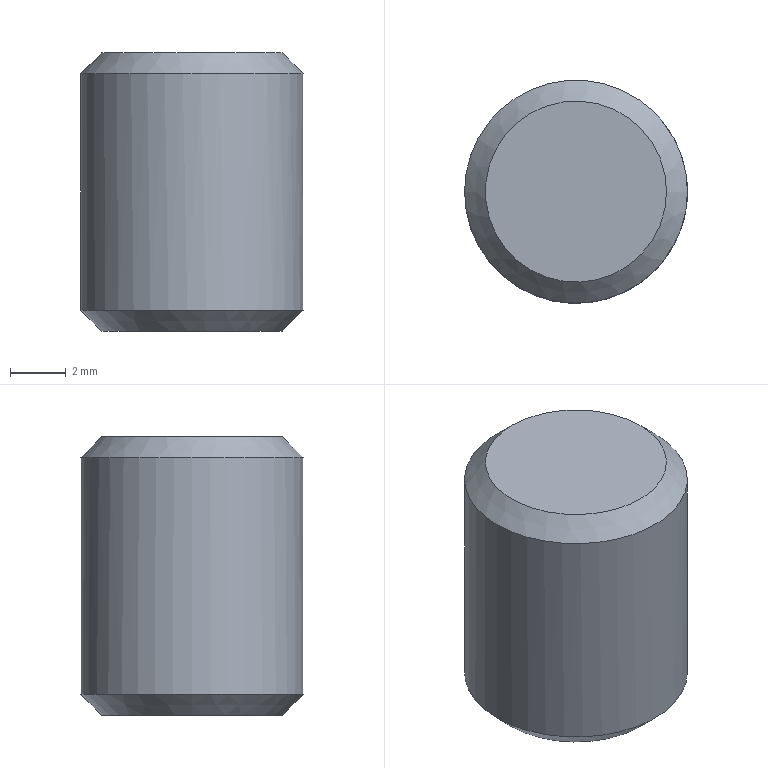Part | STEP file | 1 solid | 12 faces | box 8 x 8 x 10 mm | volume 413.018 mm3 | plane 9 | cone 2 | cylinder 1 | commonest cylinder face diameters 8 x1
STEP:
#1=CARTESIAN_POINT('',(0.,0.,0.));
#2=DIRECTION('',(0.,0.,1.));
#3=DIRECTION('',(1.,0.,0.));
#4=AXIS2_PLACEMENT_3D('',#1,#2,#3);
#5=CARTESIAN_POINT('',(1479.84,472.48,-145.381));
#6=VERTEX_POINT('',#5);
#7=CARTESIAN_POINT('',(1483.09,472.48,-145.381));
#8=DIRECTION('',(0.,0.,-1.));
#9=DIRECTION('',(-1.,0.,0.));
#10=AXIS2_PLACEMENT_3D('',#7,#8,#9);
#11=CIRCLE('',#10,3.25);
#12=CARTESIAN_POINT('',(1483.09,472.48,-145.381));
#13=DIRECTION('',(0.,0.,-1.));
#14=DIRECTION('',(-1.,0.,0.));
#15=AXIS2_PLACEMENT_3D('',#12,#13,#14);
#16=PLANE('',#15);
#17=CARTESIAN_POINT('',(0.,0.));
#18=DIRECTION('',(1.,0.));
#19=AXIS2_PLACEMENT_2D('',#17,#18);
#20=CIRCLE('',#19,3.25);
#21=(GEOMETRIC_REPRESENTATION_CONTEXT(2)PARAMETRIC_REPRESENTATION_CONTEXT()REPRESENTATION_CONTEXT('',''));
#22=DEFINITIONAL_REPRESENTATION('',(#20),#21);
#23=PCURVE('',#16,#22);
#24=CARTESIAN_POINT('',(1483.09,472.48,-144.631));
#25=DIRECTION('',(0.,0.,1.));
#26=DIRECTION('',(1.,0.,0.));
#27=AXIS2_PLACEMENT_3D('',#24,#25,#26);
#28=CONICAL_SURFACE('',#27,4.,0.7854);
#29=CARTESIAN_POINT('',(9.425,-0.75));
#30=DIRECTION('',(-1.,0.));
#31=VECTOR('',#30,1.);
#32=LINE('',#29,#31);
#33=(GEOMETRIC_REPRESENTATION_CONTEXT(2)PARAMETRIC_REPRESENTATION_CONTEXT()REPRESENTATION_CONTEXT('',''));
#34=DEFINITIONAL_REPRESENTATION('',(#32),#33);
#35=PCURVE('',#28,#34);
#36=SURFACE_CURVE('',#11,(#23,#35),.PCURVE_S1.);
#37=EDGE_CURVE('',#6,#6,#36,.T.);
#38=ORIENTED_EDGE('',*,*,#37,.T.);
#39=EDGE_LOOP('',(#38));
#40=FACE_BOUND('',#39,.T.);
#41=CARTESIAN_POINT('',(1485.19,471.268,-145.381));
#42=VERTEX_POINT('',#41);
#43=CARTESIAN_POINT('',(1483.09,470.056,-145.381));
#44=VERTEX_POINT('',#43);
#45=CARTESIAN_POINT('',(1485.19,471.268,-145.381));
#46=DIRECTION('',(-0.866,-0.5,0.));
#47=VECTOR('',#46,1.);
#48=LINE('',#45,#47);
#49=CARTESIAN_POINT('',(-2.1,-1.212));
#50=DIRECTION('',(0.866,-0.5));
#51=VECTOR('',#50,1.);
#52=LINE('',#49,#51);
#53=(GEOMETRIC_REPRESENTATION_CONTEXT(2)PARAMETRIC_REPRESENTATION_CONTEXT()REPRESENTATION_CONTEXT('',''));
#54=DEFINITIONAL_REPRESENTATION('',(#52),#53);
#55=PCURVE('',#16,#54);
#56=CARTESIAN_POINT('',(1485.19,471.268,-95.881));
#57=DIRECTION('',(0.5,-0.866,0.));
#58=DIRECTION('',(-0.866,-0.5,0.));
#59=AXIS2_PLACEMENT_3D('',#56,#57,#58);
#60=PLANE('',#59);
#61=CARTESIAN_POINT('',(0.,49.5));
#62=DIRECTION('',(1.,0.));
#63=VECTOR('',#62,1.);
#64=LINE('',#61,#63);
#65=(GEOMETRIC_REPRESENTATION_CONTEXT(2)PARAMETRIC_REPRESENTATION_CONTEXT()REPRESENTATION_CONTEXT('',''));
#66=DEFINITIONAL_REPRESENTATION('',(#64),#65);
#67=PCURVE('',#60,#66);
#68=SURFACE_CURVE('',#48,(#55,#67),.PCURVE_S1.);
#69=EDGE_CURVE('',#42,#44,#68,.T.);
#70=ORIENTED_EDGE('',*,*,#69,.F.);
#71=CARTESIAN_POINT('',(1485.19,473.693,-145.381));
#72=VERTEX_POINT('',#71);
#73=CARTESIAN_POINT('',(1485.19,473.693,-145.381));
#74=DIRECTION('',(0.,-1.,0.));
#75=VECTOR('',#74,1.);
#76=LINE('',#73,#75);
#77=CARTESIAN_POINT('',(-2.1,1.212));
#78=DIRECTION('',(0.,-1.));
#79=VECTOR('',#78,1.);
#80=LINE('',#77,#79);
#81=(GEOMETRIC_REPRESENTATION_CONTEXT(2)PARAMETRIC_REPRESENTATION_CONTEXT()REPRESENTATION_CONTEXT('',''));
#82=DEFINITIONAL_REPRESENTATION('',(#80),#81);
#83=PCURVE('',#16,#82);
#84=CARTESIAN_POINT('',(1485.19,473.693,-95.881));
#85=DIRECTION('',(1.,0.,0.));
#86=DIRECTION('',(0.,0.,-1.));
#87=AXIS2_PLACEMENT_3D('',#84,#85,#86);
#88=PLANE('',#87);
#89=CARTESIAN_POINT('',(49.5,0.));
#90=DIRECTION('',(0.,-1.));
#91=VECTOR('',#90,1.);
#92=LINE('',#89,#91);
#93=(GEOMETRIC_REPRESENTATION_CONTEXT(2)PARAMETRIC_REPRESENTATION_CONTEXT()REPRESENTATION_CONTEXT('',''));
#94=DEFINITIONAL_REPRESENTATION('',(#92),#93);
#95=PCURVE('',#88,#94);
#96=SURFACE_CURVE('',#76,(#83,#95),.PCURVE_S1.);
#97=EDGE_CURVE('',#72,#42,#96,.T.);
#98=ORIENTED_EDGE('',*,*,#97,.F.);
#99=CARTESIAN_POINT('',(1483.09,474.905,-145.381));
#100=VERTEX_POINT('',#99);
#101=CARTESIAN_POINT('',(1483.09,474.905,-145.381));
#102=DIRECTION('',(0.866,-0.5,0.));
#103=VECTOR('',#102,1.);
#104=LINE('',#101,#103);
#105=CARTESIAN_POINT('',(-0.000000005,2.425));
#106=DIRECTION('',(-0.866,-0.5));
#107=VECTOR('',#106,1.);
#108=LINE('',#105,#107);
#109=(GEOMETRIC_REPRESENTATION_CONTEXT(2)PARAMETRIC_REPRESENTATION_CONTEXT()REPRESENTATION_CONTEXT('',''));
#110=DEFINITIONAL_REPRESENTATION('',(#108),#109);
#111=PCURVE('',#16,#110);
#112=CARTESIAN_POINT('',(1483.09,474.905,-95.881));
#113=DIRECTION('',(0.5,0.866,0.));
#114=DIRECTION('',(0.866,-0.5,0.));
#115=AXIS2_PLACEMENT_3D('',#112,#113,#114);
#116=PLANE('',#115);
#117=CARTESIAN_POINT('',(0.,49.5));
#118=DIRECTION('',(1.,0.));
#119=VECTOR('',#118,1.);
#120=LINE('',#117,#119);
#121=(GEOMETRIC_REPRESENTATION_CONTEXT(2)PARAMETRIC_REPRESENTATION_CONTEXT()REPRESENTATION_CONTEXT('',''));
#122=DEFINITIONAL_REPRESENTATION('',(#120),#121);
#123=PCURVE('',#116,#122);
#124=SURFACE_CURVE('',#104,(#111,#123),.PCURVE_S1.);
#125=EDGE_CURVE('',#100,#72,#124,.T.);
#126=ORIENTED_EDGE('',*,*,#125,.F.);
#127=CARTESIAN_POINT('',(1480.99,473.693,-145.381));
#128=VERTEX_POINT('',#127);
#129=CARTESIAN_POINT('',(1480.99,473.693,-145.381));
#130=DIRECTION('',(0.866,0.5,0.));
#131=VECTOR('',#130,1.);
#132=LINE('',#129,#131);
#133=CARTESIAN_POINT('',(2.1,1.212));
#134=DIRECTION('',(-0.866,0.5));
#135=VECTOR('',#134,1.);
#136=LINE('',#133,#135);
#137=(GEOMETRIC_REPRESENTATION_CONTEXT(2)PARAMETRIC_REPRESENTATION_CONTEXT()REPRESENTATION_CONTEXT('',''));
#138=DEFINITIONAL_REPRESENTATION('',(#136),#137);
#139=PCURVE('',#16,#138);
#140=CARTESIAN_POINT('',(1480.99,473.693,-95.881));
#141=DIRECTION('',(-0.5,0.866,0.));
#142=DIRECTION('',(0.866,0.5,0.));
#143=AXIS2_PLACEMENT_3D('',#140,#141,#142);
#144=PLANE('',#143);
#145=CARTESIAN_POINT('',(0.,49.5));
#146=DIRECTION('',(1.,0.));
#147=VECTOR('',#146,1.);
#148=LINE('',#145,#147);
#149=(GEOMETRIC_REPRESENTATION_CONTEXT(2)PARAMETRIC_REPRESENTATION_CONTEXT()REPRESENTATION_CONTEXT('',''));
#150=DEFINITIONAL_REPRESENTATION('',(#148),#149);
#151=PCURVE('',#144,#150);
#152=SURFACE_CURVE('',#132,(#139,#151),.PCURVE_S1.);
#153=EDGE_CURVE('',#128,#100,#152,.T.);
#154=ORIENTED_EDGE('',*,*,#153,.F.);
#155=CARTESIAN_POINT('',(1480.99,471.268,-145.381));
#156=VERTEX_POINT('',#155);
#157=CARTESIAN_POINT('',(1480.99,471.268,-145.381));
#158=DIRECTION('',(0.,1.,0.));
#159=VECTOR('',#158,1.);
#160=LINE('',#157,#159);
#161=CARTESIAN_POINT('',(2.1,-1.212));
#162=DIRECTION('',(0.,1.));
#163=VECTOR('',#162,1.);
#164=LINE('',#161,#163);
#165=(GEOMETRIC_REPRESENTATION_CONTEXT(2)PARAMETRIC_REPRESENTATION_CONTEXT()REPRESENTATION_CONTEXT('',''));
#166=DEFINITIONAL_REPRESENTATION('',(#164),#165);
#167=PCURVE('',#16,#166);
#168=CARTESIAN_POINT('',(1480.99,471.268,-95.881));
#169=DIRECTION('',(-1.,0.,0.));
#170=DIRECTION('',(0.,0.,1.));
#171=AXIS2_PLACEMENT_3D('',#168,#169,#170);
#172=PLANE('',#171);
#173=CARTESIAN_POINT('',(-49.5,0.));
#174=DIRECTION('',(0.,1.));
#175=VECTOR('',#174,1.);
#176=LINE('',#173,#175);
#177=(GEOMETRIC_REPRESENTATION_CONTEXT(2)PARAMETRIC_REPRESENTATION_CONTEXT()REPRESENTATION_CONTEXT('',''));
#178=DEFINITIONAL_REPRESENTATION('',(#176),#177);
#179=PCURVE('',#172,#178);
#180=SURFACE_CURVE('',#160,(#167,#179),.PCURVE_S1.);
#181=EDGE_CURVE('',#156,#128,#180,.T.);
#182=ORIENTED_EDGE('',*,*,#181,.F.);
#183=CARTESIAN_POINT('',(1483.09,470.056,-145.381));
#184=DIRECTION('',(-0.866,0.5,0.));
#185=VECTOR('',#184,1.);
#186=LINE('',#183,#185);
#187=CARTESIAN_POINT('',(-0.000000005,-2.425));
#188=DIRECTION('',(0.866,0.5));
#189=VECTOR('',#188,1.);
#190=LINE('',#187,#189);
#191=(GEOMETRIC_REPRESENTATION_CONTEXT(2)PARAMETRIC_REPRESENTATION_CONTEXT()REPRESENTATION_CONTEXT('',''));
#192=DEFINITIONAL_REPRESENTATION('',(#190),#191);
#193=PCURVE('',#16,#192);
#194=CARTESIAN_POINT('',(1483.09,470.056,-95.881));
#195=DIRECTION('',(-0.5,-0.866,0.));
#196=DIRECTION('',(-0.866,0.5,0.));
#197=AXIS2_PLACEMENT_3D('',#194,#195,#196);
#198=PLANE('',#197);
#199=CARTESIAN_POINT('',(0.,49.5));
#200=DIRECTION('',(1.,0.));
#201=VECTOR('',#200,1.);
#202=LINE('',#199,#201);
#203=(GEOMETRIC_REPRESENTATION_CONTEXT(2)PARAMETRIC_REPRESENTATION_CONTEXT()REPRESENTATION_CONTEXT('',''));
#204=DEFINITIONAL_REPRESENTATION('',(#202),#203);
#205=PCURVE('',#198,#204);
#206=SURFACE_CURVE('',#186,(#193,#205),.PCURVE_S1.);
#207=EDGE_CURVE('',#44,#156,#206,.T.);
#208=ORIENTED_EDGE('',*,*,#207,.F.);
#209=EDGE_LOOP('',(#70,#98,#126,#154,#182,#208));
#210=FACE_BOUND('',#209,.T.);
#211=ADVANCED_FACE('',(#40,#210),#16,.T.);
#212=CARTESIAN_POINT('',(1486.34,472.48,-135.381));
#213=VERTEX_POINT('',#212);
#214=CARTESIAN_POINT('',(1483.09,472.48,-135.381));
#215=DIRECTION('',(0.,0.,1.));
#216=DIRECTION('',(1.,0.,0.));
#217=AXIS2_PLACEMENT_3D('',#214,#215,#216);
#218=CIRCLE('',#217,3.25);
#219=CARTESIAN_POINT('',(1483.09,472.48,-135.381));
#220=DIRECTION('',(0.,0.,1.));
#221=DIRECTION('',(1.,0.,0.));
#222=AXIS2_PLACEMENT_3D('',#219,#220,#221);
#223=PLANE('',#222);
#224=CARTESIAN_POINT('',(0.,0.));
#225=DIRECTION('',(1.,0.));
#226=AXIS2_PLACEMENT_2D('',#224,#225);
#227=CIRCLE('',#226,3.25);
#228=(GEOMETRIC_REPRESENTATION_CONTEXT(2)PARAMETRIC_REPRESENTATION_CONTEXT()REPRESENTATION_CONTEXT('',''));
#229=DEFINITIONAL_REPRESENTATION('',(#227),#228);
#230=PCURVE('',#223,#229);
#231=CARTESIAN_POINT('',(1483.09,472.48,-136.131));
#232=DIRECTION('',(0.,0.,-1.));
#233=DIRECTION('',(-1.,0.,0.));
#234=AXIS2_PLACEMENT_3D('',#231,#232,#233);
#235=CONICAL_SURFACE('',#234,4.,0.7854);
#236=CARTESIAN_POINT('',(9.425,-0.75));
#237=DIRECTION('',(-1.,0.));
#238=VECTOR('',#237,1.);
#239=LINE('',#236,#238);
#240=(GEOMETRIC_REPRESENTATION_CONTEXT(2)PARAMETRIC_REPRESENTATION_CONTEXT()REPRESENTATION_CONTEXT('',''));
#241=DEFINITIONAL_REPRESENTATION('',(#239),#240);
#242=PCURVE('',#235,#241);
#243=SURFACE_CURVE('',#218,(#230,#242),.PCURVE_S1.);
#244=EDGE_CURVE('',#213,#213,#243,.T.);
#245=ORIENTED_EDGE('',*,*,#244,.T.);
#246=EDGE_LOOP('',(#245));
#247=FACE_BOUND('',#246,.T.);
#248=ADVANCED_FACE('',(#247),#223,.T.);
#249=CARTESIAN_POINT('',(1487.09,472.48,-136.131));
#250=VERTEX_POINT('',#249);
#251=CARTESIAN_POINT('',(1479.09,472.48,-136.131));
#252=VERTEX_POINT('',#251);
#253=CARTESIAN_POINT('',(1483.09,472.48,-136.131));
#254=DIRECTION('',(0.,0.,-1.));
#255=DIRECTION('',(1.,0.,0.));
#256=AXIS2_PLACEMENT_3D('',#253,#254,#255);
#257=CIRCLE('',#256,4.);
#258=CARTESIAN_POINT('',(1483.09,472.48,-135.381));
#259=DIRECTION('',(0.,0.,-1.));
#260=DIRECTION('',(-1.,0.,0.));
#261=AXIS2_PLACEMENT_3D('',#258,#259,#260);
#262=CYLINDRICAL_SURFACE('',#261,4.);
#263=CARTESIAN_POINT('',(3.142,0.75));
#264=DIRECTION('',(1.,0.));
#265=VECTOR('',#264,1.);
#266=LINE('',#263,#265);
#267=(GEOMETRIC_REPRESENTATION_CONTEXT(2)PARAMETRIC_REPRESENTATION_CONTEXT()REPRESENTATION_CONTEXT('',''));
#268=DEFINITIONAL_REPRESENTATION('',(#266),#267);
#269=PCURVE('',#262,#268);
#270=CARTESIAN_POINT('',(3.142,0.));
#271=DIRECTION('',(1.,0.));
#272=VECTOR('',#271,1.);
#273=LINE('',#270,#272);
#274=(GEOMETRIC_REPRESENTATION_CONTEXT(2)PARAMETRIC_REPRESENTATION_CONTEXT()REPRESENTATION_CONTEXT('',''));
#275=DEFINITIONAL_REPRESENTATION('',(#273),#274);
#276=PCURVE('',#235,#275);
#277=SURFACE_CURVE('',#257,(#269,#276),.PCURVE_S1.);
#278=EDGE_CURVE('',#250,#252,#277,.T.);
#279=ORIENTED_EDGE('',*,*,#278,.T.);
#280=CARTESIAN_POINT('',(1479.09,472.48,-144.631));
#281=VERTEX_POINT('',#280);
#282=CARTESIAN_POINT('',(1479.09,472.48,-136.131));
#283=CARTESIAN_POINT('',(1479.09,472.48,-144.631));
#284=B_SPLINE_CURVE_WITH_KNOTS('',1,(#282,#283),.UNSPECIFIED.,.F.,.F.,(2,2),(0.75,9.25),.PIECEWISE_BEZIER_KNOTS.);
#285=CARTESIAN_POINT('',(6.283,0.));
#286=DIRECTION('',(0.,1.));
#287=VECTOR('',#286,1.);
#288=LINE('',#285,#287);
#289=(GEOMETRIC_REPRESENTATION_CONTEXT(2)PARAMETRIC_REPRESENTATION_CONTEXT()REPRESENTATION_CONTEXT('',''));
#290=DEFINITIONAL_REPRESENTATION('',(#288),#289);
#291=PCURVE('',#262,#290);
#292=CARTESIAN_POINT('',(0.,0.));
#293=DIRECTION('',(0.,1.));
#294=VECTOR('',#293,1.);
#295=LINE('',#292,#294);
#296=(GEOMETRIC_REPRESENTATION_CONTEXT(2)PARAMETRIC_REPRESENTATION_CONTEXT()REPRESENTATION_CONTEXT('',''));
#297=DEFINITIONAL_REPRESENTATION('',(#295),#296);
#298=PCURVE('',#262,#297);
#299=SEAM_CURVE('',#284,(#291,#298),.PCURVE_S1.);
#300=EDGE_CURVE('',#252,#281,#299,.T.);
#301=ORIENTED_EDGE('',*,*,#300,.T.);
#302=CARTESIAN_POINT('',(1483.09,472.48,-144.631));
#303=DIRECTION('',(0.,0.,1.));
#304=DIRECTION('',(-1.,0.,0.));
#305=AXIS2_PLACEMENT_3D('',#302,#303,#304);
#306=CIRCLE('',#305,4.);
#307=CARTESIAN_POINT('',(6.283,9.25));
#308=DIRECTION('',(-1.,0.));
#309=VECTOR('',#308,1.);
#310=LINE('',#307,#309);
#311=(GEOMETRIC_REPRESENTATION_CONTEXT(2)PARAMETRIC_REPRESENTATION_CONTEXT()REPRESENTATION_CONTEXT('',''));
#312=DEFINITIONAL_REPRESENTATION('',(#310),#311);
#313=PCURVE('',#262,#312);
#314=CARTESIAN_POINT('',(3.142,0.));
#315=DIRECTION('',(1.,0.));
#316=VECTOR('',#315,1.);
#317=LINE('',#314,#316);
#318=(GEOMETRIC_REPRESENTATION_CONTEXT(2)PARAMETRIC_REPRESENTATION_CONTEXT()REPRESENTATION_CONTEXT('',''));
#319=DEFINITIONAL_REPRESENTATION('',(#317),#318);
#320=PCURVE('',#28,#319);
#321=SURFACE_CURVE('',#306,(#313,#320),.PCURVE_S1.);
#322=EDGE_CURVE('',#281,#281,#321,.T.);
#323=ORIENTED_EDGE('',*,*,#322,.T.);
#324=ORIENTED_EDGE('',*,*,#300,.F.);
#325=CARTESIAN_POINT('',(1483.09,472.48,-136.131));
#326=DIRECTION('',(0.,0.,-1.));
#327=DIRECTION('',(1.,0.,0.));
#328=AXIS2_PLACEMENT_3D('',#325,#326,#327);
#329=CIRCLE('',#328,4.);
#330=CARTESIAN_POINT('',(-3.142,0.75));
#331=DIRECTION('',(1.,0.));
#332=VECTOR('',#331,1.);
#333=LINE('',#330,#332);
#334=(GEOMETRIC_REPRESENTATION_CONTEXT(2)PARAMETRIC_REPRESENTATION_CONTEXT()REPRESENTATION_CONTEXT('',''));
#335=DEFINITIONAL_REPRESENTATION('',(#333),#334);
#336=PCURVE('',#262,#335);
#337=CARTESIAN_POINT('',(3.142,0.));
#338=DIRECTION('',(1.,0.));
#339=VECTOR('',#338,1.);
#340=LINE('',#337,#339);
#341=(GEOMETRIC_REPRESENTATION_CONTEXT(2)PARAMETRIC_REPRESENTATION_CONTEXT()REPRESENTATION_CONTEXT('',''));
#342=DEFINITIONAL_REPRESENTATION('',(#340),#341);
#343=PCURVE('',#235,#342);
#344=SURFACE_CURVE('',#329,(#336,#343),.PCURVE_S1.);
#345=EDGE_CURVE('',#252,#250,#344,.T.);
#346=ORIENTED_EDGE('',*,*,#345,.T.);
#347=EDGE_LOOP('',(#279,#301,#323,#324,#346));
#348=FACE_BOUND('',#347,.T.);
#349=ADVANCED_FACE('',(#348),#262,.T.);
#350=CARTESIAN_POINT('',(1485.19,471.268,-140.381));
#351=VERTEX_POINT('',#350);
#352=CARTESIAN_POINT('',(1483.09,470.056,-140.381));
#353=VERTEX_POINT('',#352);
#354=CARTESIAN_POINT('',(1485.19,471.268,-140.381));
#355=DIRECTION('',(-0.866,-0.5,0.));
#356=VECTOR('',#355,1.);
#357=LINE('',#354,#356);
#358=CARTESIAN_POINT('',(-15517.929,4465.25,-140.381));
#359=DIRECTION('',(0.,0.,-1.));
#360=DIRECTION('',(-1.,0.,0.));
#361=AXIS2_PLACEMENT_3D('',#358,#359,#360);
#362=PLANE('',#361);
#363=CARTESIAN_POINT('',(-17003.119,-3993.982));
#364=DIRECTION('',(0.866,-0.5));
#365=VECTOR('',#364,1.);
#366=LINE('',#363,#365);
#367=(GEOMETRIC_REPRESENTATION_CONTEXT(2)PARAMETRIC_REPRESENTATION_CONTEXT()REPRESENTATION_CONTEXT('',''));
#368=DEFINITIONAL_REPRESENTATION('',(#366),#367);
#369=PCURVE('',#362,#368);
#370=CARTESIAN_POINT('',(0.,44.5));
#371=DIRECTION('',(1.,0.));
#372=VECTOR('',#371,1.);
#373=LINE('',#370,#372);
#374=(GEOMETRIC_REPRESENTATION_CONTEXT(2)PARAMETRIC_REPRESENTATION_CONTEXT()REPRESENTATION_CONTEXT('',''));
#375=DEFINITIONAL_REPRESENTATION('',(#373),#374);
#376=PCURVE('',#60,#375);
#377=SURFACE_CURVE('',#357,(#369,#376),.PCURVE_S1.);
#378=EDGE_CURVE('',#351,#353,#377,.T.);
#379=ORIENTED_EDGE('',*,*,#378,.T.);
#380=CARTESIAN_POINT('',(1480.99,471.268,-140.381));
#381=VERTEX_POINT('',#380);
#382=CARTESIAN_POINT('',(1483.09,470.056,-140.381));
#383=DIRECTION('',(-0.866,0.5,0.));
#384=VECTOR('',#383,1.);
#385=LINE('',#382,#384);
#386=CARTESIAN_POINT('',(-17001.019,-3995.194));
#387=DIRECTION('',(0.866,0.5));
#388=VECTOR('',#387,1.);
#389=LINE('',#386,#388);
#390=(GEOMETRIC_REPRESENTATION_CONTEXT(2)PARAMETRIC_REPRESENTATION_CONTEXT()REPRESENTATION_CONTEXT('',''));
#391=DEFINITIONAL_REPRESENTATION('',(#389),#390);
#392=PCURVE('',#362,#391);
#393=CARTESIAN_POINT('',(0.,44.5));
#394=DIRECTION('',(1.,0.));
#395=VECTOR('',#394,1.);
#396=LINE('',#393,#395);
#397=(GEOMETRIC_REPRESENTATION_CONTEXT(2)PARAMETRIC_REPRESENTATION_CONTEXT()REPRESENTATION_CONTEXT('',''));
#398=DEFINITIONAL_REPRESENTATION('',(#396),#397);
#399=PCURVE('',#198,#398);
#400=SURFACE_CURVE('',#385,(#392,#399),.PCURVE_S1.);
#401=EDGE_CURVE('',#353,#381,#400,.T.);
#402=ORIENTED_EDGE('',*,*,#401,.T.);
#403=CARTESIAN_POINT('',(1480.99,473.693,-140.381));
#404=VERTEX_POINT('',#403);
#405=CARTESIAN_POINT('',(1480.99,471.268,-140.381));
#406=DIRECTION('',(0.,1.,0.));
#407=VECTOR('',#406,1.);
#408=LINE('',#405,#407);
#409=CARTESIAN_POINT('',(-16998.919,-3993.982));
#410=DIRECTION('',(0.,1.));
#411=VECTOR('',#410,1.);
#412=LINE('',#409,#411);
#413=(GEOMETRIC_REPRESENTATION_CONTEXT(2)PARAMETRIC_REPRESENTATION_CONTEXT()REPRESENTATION_CONTEXT('',''));
#414=DEFINITIONAL_REPRESENTATION('',(#412),#413);
#415=PCURVE('',#362,#414);
#416=CARTESIAN_POINT('',(-44.5,0.));
#417=DIRECTION('',(0.,1.));
#418=VECTOR('',#417,1.);
#419=LINE('',#416,#418);
#420=(GEOMETRIC_REPRESENTATION_CONTEXT(2)PARAMETRIC_REPRESENTATION_CONTEXT()REPRESENTATION_CONTEXT('',''));
#421=DEFINITIONAL_REPRESENTATION('',(#419),#420);
#422=PCURVE('',#172,#421);
#423=SURFACE_CURVE('',#408,(#415,#422),.PCURVE_S1.);
#424=EDGE_CURVE('',#381,#404,#423,.T.);
#425=ORIENTED_EDGE('',*,*,#424,.T.);
#426=CARTESIAN_POINT('',(1483.09,474.905,-140.381));
#427=VERTEX_POINT('',#426);
#428=CARTESIAN_POINT('',(1480.99,473.693,-140.381));
#429=DIRECTION('',(0.866,0.5,0.));
#430=VECTOR('',#429,1.);
#431=LINE('',#428,#430);
#432=CARTESIAN_POINT('',(-16998.919,-3991.557));
#433=DIRECTION('',(-0.866,0.5));
#434=VECTOR('',#433,1.);
#435=LINE('',#432,#434);
#436=(GEOMETRIC_REPRESENTATION_CONTEXT(2)PARAMETRIC_REPRESENTATION_CONTEXT()REPRESENTATION_CONTEXT('',''));
#437=DEFINITIONAL_REPRESENTATION('',(#435),#436);
#438=PCURVE('',#362,#437);
#439=CARTESIAN_POINT('',(0.,44.5));
#440=DIRECTION('',(1.,0.));
#441=VECTOR('',#440,1.);
#442=LINE('',#439,#441);
#443=(GEOMETRIC_REPRESENTATION_CONTEXT(2)PARAMETRIC_REPRESENTATION_CONTEXT()REPRESENTATION_CONTEXT('',''));
#444=DEFINITIONAL_REPRESENTATION('',(#442),#443);
#445=PCURVE('',#144,#444);
#446=SURFACE_CURVE('',#431,(#438,#445),.PCURVE_S1.);
#447=EDGE_CURVE('',#404,#427,#446,.T.);
#448=ORIENTED_EDGE('',*,*,#447,.T.);
#449=CARTESIAN_POINT('',(1485.19,473.693,-140.381));
#450=VERTEX_POINT('',#449);
#451=CARTESIAN_POINT('',(1483.09,474.905,-140.381));
#452=DIRECTION('',(0.866,-0.5,0.));
#453=VECTOR('',#452,1.);
#454=LINE('',#451,#453);
#455=CARTESIAN_POINT('',(-17001.019,-3990.344));
#456=DIRECTION('',(-0.866,-0.5));
#457=VECTOR('',#456,1.);
#458=LINE('',#455,#457);
#459=(GEOMETRIC_REPRESENTATION_CONTEXT(2)PARAMETRIC_REPRESENTATION_CONTEXT()REPRESENTATION_CONTEXT('',''));
#460=DEFINITIONAL_REPRESENTATION('',(#458),#459);
#461=PCURVE('',#362,#460);
#462=CARTESIAN_POINT('',(0.,44.5));
#463=DIRECTION('',(1.,0.));
#464=VECTOR('',#463,1.);
#465=LINE('',#462,#464);
#466=(GEOMETRIC_REPRESENTATION_CONTEXT(2)PARAMETRIC_REPRESENTATION_CONTEXT()REPRESENTATION_CONTEXT('',''));
#467=DEFINITIONAL_REPRESENTATION('',(#465),#466);
#468=PCURVE('',#116,#467);
#469=SURFACE_CURVE('',#454,(#461,#468),.PCURVE_S1.);
#470=EDGE_CURVE('',#427,#450,#469,.T.);
#471=ORIENTED_EDGE('',*,*,#470,.T.);
#472=CARTESIAN_POINT('',(1485.19,473.693,-140.381));
#473=DIRECTION('',(0.,-1.,0.));
#474=VECTOR('',#473,1.);
#475=LINE('',#472,#474);
#476=CARTESIAN_POINT('',(-17003.119,-3991.557));
#477=DIRECTION('',(0.,-1.));
#478=VECTOR('',#477,1.);
#479=LINE('',#476,#478);
#480=(GEOMETRIC_REPRESENTATION_CONTEXT(2)PARAMETRIC_REPRESENTATION_CONTEXT()REPRESENTATION_CONTEXT('',''));
#481=DEFINITIONAL_REPRESENTATION('',(#479),#480);
#482=PCURVE('',#362,#481);
#483=CARTESIAN_POINT('',(44.5,0.));
#484=DIRECTION('',(0.,-1.));
#485=VECTOR('',#484,1.);
#486=LINE('',#483,#485);
#487=(GEOMETRIC_REPRESENTATION_CONTEXT(2)PARAMETRIC_REPRESENTATION_CONTEXT()REPRESENTATION_CONTEXT('',''));
#488=DEFINITIONAL_REPRESENTATION('',(#486),#487);
#489=PCURVE('',#88,#488);
#490=SURFACE_CURVE('',#475,(#482,#489),.PCURVE_S1.);
#491=EDGE_CURVE('',#450,#351,#490,.T.);
#492=ORIENTED_EDGE('',*,*,#491,.T.);
#493=EDGE_LOOP('',(#379,#402,#425,#448,#471,#492));
#494=FACE_BOUND('',#493,.T.);
#495=ADVANCED_FACE('',(#494),#362,.T.);
#496=ORIENTED_EDGE('',*,*,#378,.F.);
#497=CARTESIAN_POINT('',(1485.19,471.268,-95.881));
#498=DIRECTION('',(0.,0.,1.));
#499=VECTOR('',#498,1.);
#500=LINE('',#497,#499);
#501=CARTESIAN_POINT('',(0.,0.));
#502=DIRECTION('',(0.,-1.));
#503=VECTOR('',#502,1.);
#504=LINE('',#501,#503);
#505=(GEOMETRIC_REPRESENTATION_CONTEXT(2)PARAMETRIC_REPRESENTATION_CONTEXT()REPRESENTATION_CONTEXT('',''));
#506=DEFINITIONAL_REPRESENTATION('',(#504),#505);
#507=PCURVE('',#60,#506);
#508=CARTESIAN_POINT('',(0.,-2.425));
#509=DIRECTION('',(-1.,0.));
#510=VECTOR('',#509,1.);
#511=LINE('',#508,#510);
#512=(GEOMETRIC_REPRESENTATION_CONTEXT(2)PARAMETRIC_REPRESENTATION_CONTEXT()REPRESENTATION_CONTEXT('',''));
#513=DEFINITIONAL_REPRESENTATION('',(#511),#512);
#514=PCURVE('',#88,#513);
#515=SURFACE_CURVE('',#500,(#507,#514),.PCURVE_S1.);
#516=EDGE_CURVE('',#42,#351,#515,.T.);
#517=ORIENTED_EDGE('',*,*,#516,.F.);
#518=ORIENTED_EDGE('',*,*,#69,.T.);
#519=CARTESIAN_POINT('',(1483.09,470.056,-95.881));
#520=DIRECTION('',(0.,0.,1.));
#521=VECTOR('',#520,1.);
#522=LINE('',#519,#521);
#523=CARTESIAN_POINT('',(2.425,0.));
#524=DIRECTION('',(0.,-1.));
#525=VECTOR('',#524,1.);
#526=LINE('',#523,#525);
#527=(GEOMETRIC_REPRESENTATION_CONTEXT(2)PARAMETRIC_REPRESENTATION_CONTEXT()REPRESENTATION_CONTEXT('',''));
#528=DEFINITIONAL_REPRESENTATION('',(#526),#527);
#529=PCURVE('',#60,#528);
#530=CARTESIAN_POINT('',(0.,0.));
#531=DIRECTION('',(0.,-1.));
#532=VECTOR('',#531,1.);
#533=LINE('',#530,#532);
#534=(GEOMETRIC_REPRESENTATION_CONTEXT(2)PARAMETRIC_REPRESENTATION_CONTEXT()REPRESENTATION_CONTEXT('',''));
#535=DEFINITIONAL_REPRESENTATION('',(#533),#534);
#536=PCURVE('',#198,#535);
#537=SURFACE_CURVE('',#522,(#529,#536),.PCURVE_S1.);
#538=EDGE_CURVE('',#44,#353,#537,.T.);
#539=ORIENTED_EDGE('',*,*,#538,.T.);
#540=EDGE_LOOP('',(#496,#517,#518,#539));
#541=FACE_BOUND('',#540,.T.);
#542=ADVANCED_FACE('',(#541),#60,.F.);
#543=ORIENTED_EDGE('',*,*,#401,.F.);
#544=ORIENTED_EDGE('',*,*,#538,.F.);
#545=ORIENTED_EDGE('',*,*,#207,.T.);
#546=CARTESIAN_POINT('',(1480.99,471.268,-95.881));
#547=DIRECTION('',(0.,0.,1.));
#548=VECTOR('',#547,1.);
#549=LINE('',#546,#548);
#550=CARTESIAN_POINT('',(2.425,0.));
#551=DIRECTION('',(0.,-1.));
#552=VECTOR('',#551,1.);
#553=LINE('',#550,#552);
#554=(GEOMETRIC_REPRESENTATION_CONTEXT(2)PARAMETRIC_REPRESENTATION_CONTEXT()REPRESENTATION_CONTEXT('',''));
#555=DEFINITIONAL_REPRESENTATION('',(#553),#554);
#556=PCURVE('',#198,#555);
#557=CARTESIAN_POINT('',(0.,0.));
#558=DIRECTION('',(1.,0.));
#559=VECTOR('',#558,1.);
#560=LINE('',#557,#559);
#561=(GEOMETRIC_REPRESENTATION_CONTEXT(2)PARAMETRIC_REPRESENTATION_CONTEXT()REPRESENTATION_CONTEXT('',''));
#562=DEFINITIONAL_REPRESENTATION('',(#560),#561);
#563=PCURVE('',#172,#562);
#564=SURFACE_CURVE('',#549,(#556,#563),.PCURVE_S1.);
#565=EDGE_CURVE('',#156,#381,#564,.T.);
#566=ORIENTED_EDGE('',*,*,#565,.T.);
#567=EDGE_LOOP('',(#543,#544,#545,#566));
#568=FACE_BOUND('',#567,.T.);
#569=ADVANCED_FACE('',(#568),#198,.F.);
#570=ORIENTED_EDGE('',*,*,#424,.F.);
#571=ORIENTED_EDGE('',*,*,#565,.F.);
#572=ORIENTED_EDGE('',*,*,#181,.T.);
#573=CARTESIAN_POINT('',(1480.99,473.693,-95.881));
#574=DIRECTION('',(0.,0.,1.));
#575=VECTOR('',#574,1.);
#576=LINE('',#573,#575);
#577=CARTESIAN_POINT('',(0.,2.425));
#578=DIRECTION('',(1.,0.));
#579=VECTOR('',#578,1.);
#580=LINE('',#577,#579);
#581=(GEOMETRIC_REPRESENTATION_CONTEXT(2)PARAMETRIC_REPRESENTATION_CONTEXT()REPRESENTATION_CONTEXT('',''));
#582=DEFINITIONAL_REPRESENTATION('',(#580),#581);
#583=PCURVE('',#172,#582);
#584=CARTESIAN_POINT('',(0.,0.));
#585=DIRECTION('',(0.,-1.));
#586=VECTOR('',#585,1.);
#587=LINE('',#584,#586);
#588=(GEOMETRIC_REPRESENTATION_CONTEXT(2)PARAMETRIC_REPRESENTATION_CONTEXT()REPRESENTATION_CONTEXT('',''));
#589=DEFINITIONAL_REPRESENTATION('',(#587),#588);
#590=PCURVE('',#144,#589);
#591=SURFACE_CURVE('',#576,(#583,#590),.PCURVE_S1.);
#592=EDGE_CURVE('',#128,#404,#591,.T.);
#593=ORIENTED_EDGE('',*,*,#592,.T.);
#594=EDGE_LOOP('',(#570,#571,#572,#593));
#595=FACE_BOUND('',#594,.T.);
#596=ADVANCED_FACE('',(#595),#172,.F.);
#597=ORIENTED_EDGE('',*,*,#447,.F.);
#598=ORIENTED_EDGE('',*,*,#592,.F.);
#599=ORIENTED_EDGE('',*,*,#153,.T.);
#600=CARTESIAN_POINT('',(1483.09,474.905,-95.881));
#601=DIRECTION('',(0.,0.,1.));
#602=VECTOR('',#601,1.);
#603=LINE('',#600,#602);
#604=CARTESIAN_POINT('',(2.425,0.));
#605=DIRECTION('',(0.,-1.));
#606=VECTOR('',#605,1.);
#607=LINE('',#604,#606);
#608=(GEOMETRIC_REPRESENTATION_CONTEXT(2)PARAMETRIC_REPRESENTATION_CONTEXT()REPRESENTATION_CONTEXT('',''));
#609=DEFINITIONAL_REPRESENTATION('',(#607),#608);
#610=PCURVE('',#144,#609);
#611=CARTESIAN_POINT('',(0.,0.));
#612=DIRECTION('',(0.,-1.));
#613=VECTOR('',#612,1.);
#614=LINE('',#611,#613);
#615=(GEOMETRIC_REPRESENTATION_CONTEXT(2)PARAMETRIC_REPRESENTATION_CONTEXT()REPRESENTATION_CONTEXT('',''));
#616=DEFINITIONAL_REPRESENTATION('',(#614),#615);
#617=PCURVE('',#116,#616);
#618=SURFACE_CURVE('',#603,(#610,#617),.PCURVE_S1.);
#619=EDGE_CURVE('',#100,#427,#618,.T.);
#620=ORIENTED_EDGE('',*,*,#619,.T.);
#621=EDGE_LOOP('',(#597,#598,#599,#620));
#622=FACE_BOUND('',#621,.T.);
#623=ADVANCED_FACE('',(#622),#144,.F.);
#624=ORIENTED_EDGE('',*,*,#470,.F.);
#625=ORIENTED_EDGE('',*,*,#619,.F.);
#626=ORIENTED_EDGE('',*,*,#125,.T.);
#627=CARTESIAN_POINT('',(1485.19,473.693,-95.881));
#628=DIRECTION('',(0.,0.,1.));
#629=VECTOR('',#628,1.);
#630=LINE('',#627,#629);
#631=CARTESIAN_POINT('',(2.425,0.));
#632=DIRECTION('',(0.,-1.));
#633=VECTOR('',#632,1.);
#634=LINE('',#631,#633);
#635=(GEOMETRIC_REPRESENTATION_CONTEXT(2)PARAMETRIC_REPRESENTATION_CONTEXT()REPRESENTATION_CONTEXT('',''));
#636=DEFINITIONAL_REPRESENTATION('',(#634),#635);
#637=PCURVE('',#116,#636);
#638=CARTESIAN_POINT('',(0.,0.));
#639=DIRECTION('',(-1.,0.));
#640=VECTOR('',#639,1.);
#641=LINE('',#638,#640);
#642=(GEOMETRIC_REPRESENTATION_CONTEXT(2)PARAMETRIC_REPRESENTATION_CONTEXT()REPRESENTATION_CONTEXT('',''));
#643=DEFINITIONAL_REPRESENTATION('',(#641),#642);
#644=PCURVE('',#88,#643);
#645=SURFACE_CURVE('',#630,(#637,#644),.PCURVE_S1.);
#646=EDGE_CURVE('',#72,#450,#645,.T.);
#647=ORIENTED_EDGE('',*,*,#646,.T.);
#648=EDGE_LOOP('',(#624,#625,#626,#647));
#649=FACE_BOUND('',#648,.T.);
#650=ADVANCED_FACE('',(#649),#116,.F.);
#651=ORIENTED_EDGE('',*,*,#491,.F.);
#652=ORIENTED_EDGE('',*,*,#646,.F.);
#653=ORIENTED_EDGE('',*,*,#97,.T.);
#654=ORIENTED_EDGE('',*,*,#516,.T.);
#655=EDGE_LOOP('',(#651,#652,#653,#654));
#656=FACE_BOUND('',#655,.T.);
#657=ADVANCED_FACE('',(#656),#88,.F.);
#658=ORIENTED_EDGE('',*,*,#244,.F.);
#659=CARTESIAN_POINT('',(1486.34,472.48,-135.381));
#660=CARTESIAN_POINT('',(1487.09,472.48,-136.131));
#661=B_SPLINE_CURVE_WITH_KNOTS('',1,(#659,#660),.UNSPECIFIED.,.F.,.F.,(2,2),(-1.061,0.),.PIECEWISE_BEZIER_KNOTS.);
#662=CARTESIAN_POINT('',(9.425,0.));
#663=DIRECTION('',(0.,1.));
#664=VECTOR('',#663,1.);
#665=LINE('',#662,#664);
#666=(GEOMETRIC_REPRESENTATION_CONTEXT(2)PARAMETRIC_REPRESENTATION_CONTEXT()REPRESENTATION_CONTEXT('',''));
#667=DEFINITIONAL_REPRESENTATION('',(#665),#666);
#668=PCURVE('',#235,#667);
#669=CARTESIAN_POINT('',(3.142,0.));
#670=DIRECTION('',(0.,1.));
#671=VECTOR('',#670,1.);
#672=LINE('',#669,#671);
#673=(GEOMETRIC_REPRESENTATION_CONTEXT(2)PARAMETRIC_REPRESENTATION_CONTEXT()REPRESENTATION_CONTEXT('',''));
#674=DEFINITIONAL_REPRESENTATION('',(#672),#673);
#675=PCURVE('',#235,#674);
#676=SEAM_CURVE('',#661,(#668,#675),.PCURVE_S1.);
#677=EDGE_CURVE('',#213,#250,#676,.T.);
#678=ORIENTED_EDGE('',*,*,#677,.T.);
#679=ORIENTED_EDGE('',*,*,#345,.F.);
#680=ORIENTED_EDGE('',*,*,#278,.F.);
#681=ORIENTED_EDGE('',*,*,#677,.F.);
#682=EDGE_LOOP('',(#658,#678,#679,#680,#681));
#683=FACE_BOUND('',#682,.T.);
#684=ADVANCED_FACE('',(#683),#235,.T.);
#685=ORIENTED_EDGE('',*,*,#37,.F.);
#686=CARTESIAN_POINT('',(1479.84,472.48,-145.381));
#687=CARTESIAN_POINT('',(1479.09,472.48,-144.631));
#688=B_SPLINE_CURVE_WITH_KNOTS('',1,(#686,#687),.UNSPECIFIED.,.F.,.F.,(2,2),(-1.061,0.),.PIECEWISE_BEZIER_KNOTS.);
#689=CARTESIAN_POINT('',(9.425,0.));
#690=DIRECTION('',(0.,1.));
#691=VECTOR('',#690,1.);
#692=LINE('',#689,#691);
#693=(GEOMETRIC_REPRESENTATION_CONTEXT(2)PARAMETRIC_REPRESENTATION_CONTEXT()REPRESENTATION_CONTEXT('',''));
#694=DEFINITIONAL_REPRESENTATION('',(#692),#693);
#695=PCURVE('',#28,#694);
#696=CARTESIAN_POINT('',(3.142,0.));
#697=DIRECTION('',(0.,1.));
#698=VECTOR('',#697,1.);
#699=LINE('',#696,#698);
#700=(GEOMETRIC_REPRESENTATION_CONTEXT(2)PARAMETRIC_REPRESENTATION_CONTEXT()REPRESENTATION_CONTEXT('',''));
#701=DEFINITIONAL_REPRESENTATION('',(#699),#700);
#702=PCURVE('',#28,#701);
#703=SEAM_CURVE('',#688,(#695,#702),.PCURVE_S1.);
#704=EDGE_CURVE('',#6,#281,#703,.T.);
#705=ORIENTED_EDGE('',*,*,#704,.T.);
#706=ORIENTED_EDGE('',*,*,#322,.F.);
#707=ORIENTED_EDGE('',*,*,#704,.F.);
#708=EDGE_LOOP('',(#685,#705,#706,#707));
#709=FACE_BOUND('',#708,.T.);
#710=ADVANCED_FACE('',(#709),#28,.T.);
#711=CLOSED_SHELL('',(#211,#248,#349,#495,#542,#569,#596,#623,#650,#657,#684,#710));
#712=MANIFOLD_SOLID_BREP('',#711);
#713=(LENGTH_UNIT()NAMED_UNIT(*)SI_UNIT(.MILLI.,.METRE.));
#714=UNCERTAINTY_MEASURE_WITH_UNIT(LENGTH_MEASURE(0.000002),#713,'','');
#715=(NAMED_UNIT(*)PLANE_ANGLE_UNIT()SI_UNIT($,.RADIAN.));
#716=(NAMED_UNIT(*)SI_UNIT($,.STERADIAN.)SOLID_ANGLE_UNIT());
#717=(GEOMETRIC_REPRESENTATION_CONTEXT(3)GLOBAL_UNCERTAINTY_ASSIGNED_CONTEXT((#714))GLOBAL_UNIT_ASSIGNED_CONTEXT((#713,#715,#716))REPRESENTATION_CONTEXT('',''));
#718=ADVANCED_BREP_SHAPE_REPRESENTATION('',(#4,#712),#717);